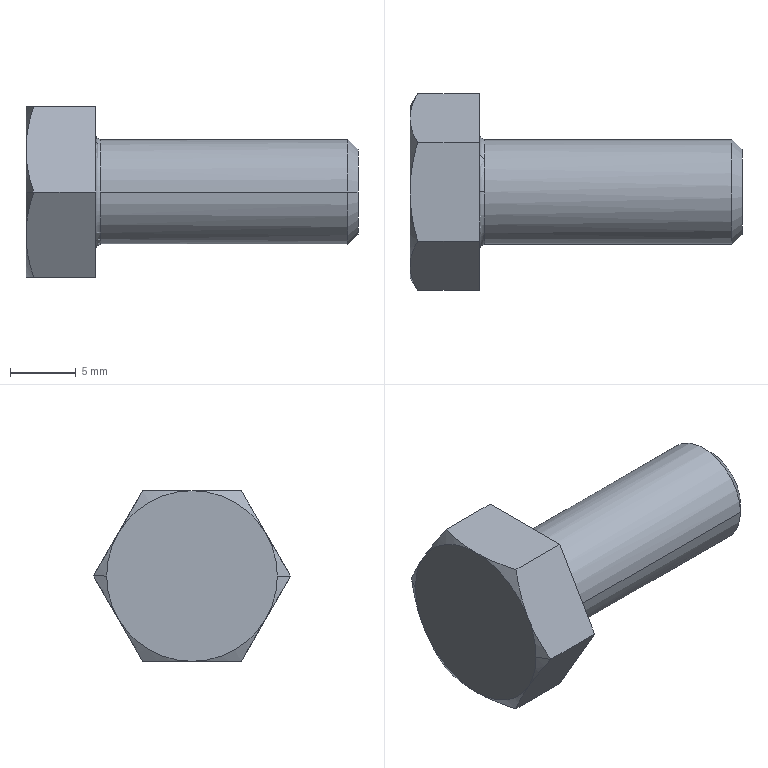Part | STEP file | KS B 1002 - C  M 8 x 20 | 1 solid | 23 faces | box 25.3 x 15.011 x 13 mm | volume 1773 mm3 | cone 10 | plane 9 | torus 2 | cylinder 2 | commonest cylinder face diameters 8 x2